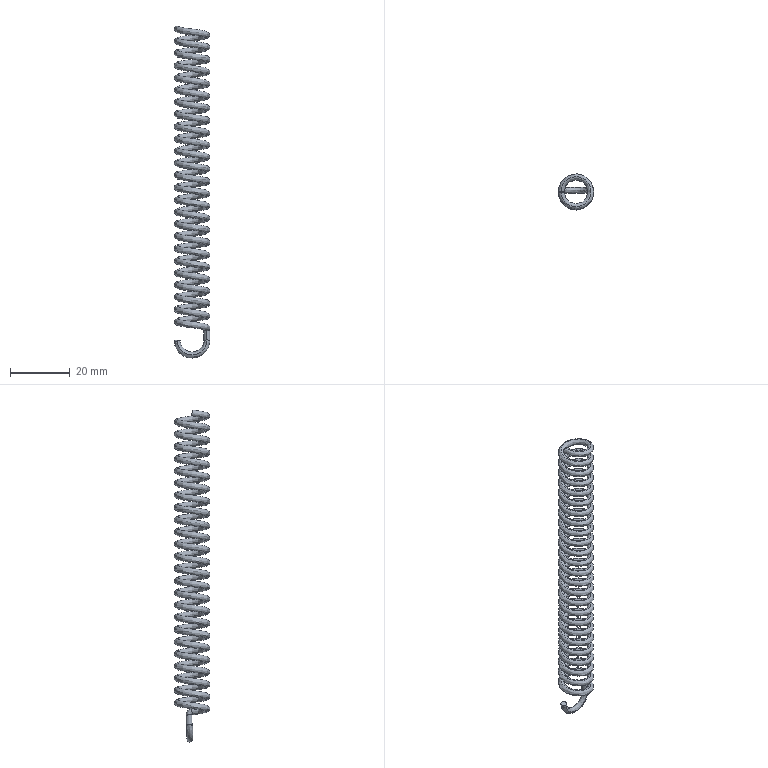Part | SolidWorks | features Sweep 3, Helix 1, MirrorPattern 1, RefAxis 1 | 1 solid | 12 faces | box 12 x 12 x 111.085 mm | volume 2504 mm3 | spline 8 | plane 4